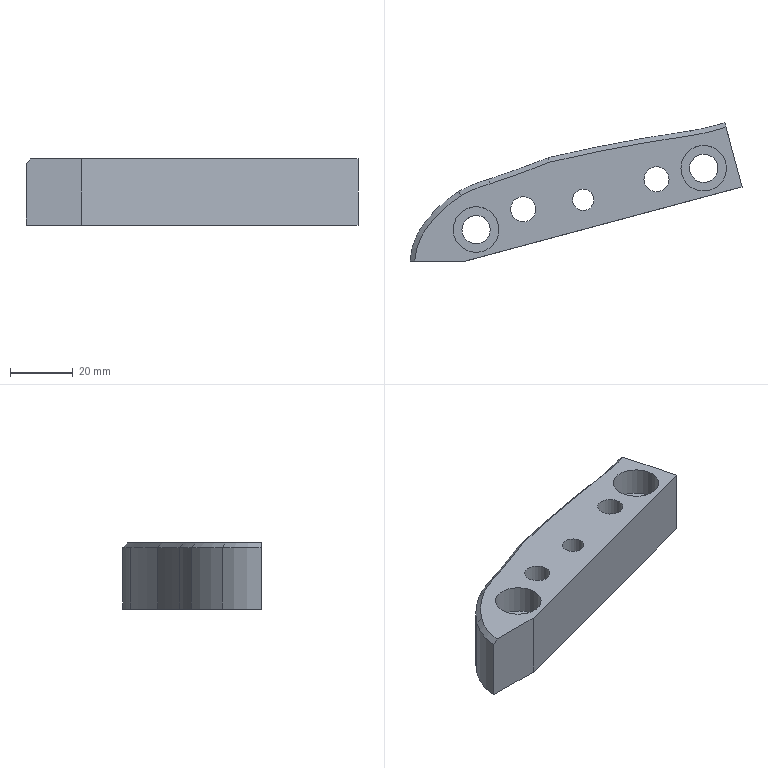Part | NX | features 23 2 | 1 solid | 26 faces | box 105.513 x 43.92 x 21 mm | volume 41296 mm3 | cylinder 13 | plane 7 | cone 6 | commonest cylinder face diameters 8.001 x2 9 x2 14.5 x2 6.8 x1 42.851 x1 79.35 x1
STEP:
#1=CARTESIAN_POINT('',(1132.197,150.506,-2.5));
#2=VERTEX_POINT('',#1);
#3=CARTESIAN_POINT('',(1124.947,150.506,-2.5));
#4=DIRECTION('',(0.,0.,1.));
#5=DIRECTION('',(1.,0.,0.));
#6=AXIS2_PLACEMENT_3D('',#3,#4,#5);
#7=CIRCLE('',#6,7.25);
#8=EDGE_CURVE('',#2,#2,#7,.T.);
#9=ORIENTED_EDGE('',*,*,#8,.F.);
#10=EDGE_LOOP('',(#9));
#11=FACE_BOUND('',#10,.T.);
#12=CARTESIAN_POINT('',(1113.947,147.035,-2.5));
#13=VERTEX_POINT('',#12);
#14=CARTESIAN_POINT('',(1109.947,147.035,-2.5));
#15=DIRECTION('',(0.,0.,-1.));
#16=DIRECTION('',(1.,0.,0.));
#17=AXIS2_PLACEMENT_3D('',#14,#15,#16);
#18=CIRCLE('',#17,4.);
#19=EDGE_CURVE('',#13,#13,#18,.T.);
#20=ORIENTED_EDGE('',*,*,#19,.T.);
#21=EDGE_LOOP('',(#20));
#22=FACE_BOUND('',#21,.T.);
#23=CARTESIAN_POINT('',(1071.605,137.506,-2.5));
#24=VERTEX_POINT('',#23);
#25=CARTESIAN_POINT('',(1067.604,137.506,-2.5));
#26=DIRECTION('',(0.,0.,-1.));
#27=DIRECTION('',(1.,0.,0.));
#28=AXIS2_PLACEMENT_3D('',#25,#26,#27);
#29=CIRCLE('',#28,4.);
#30=EDGE_CURVE('',#24,#24,#29,.T.);
#31=ORIENTED_EDGE('',*,*,#30,.T.);
#32=EDGE_LOOP('',(#31));
#33=FACE_BOUND('',#32,.T.);
#34=CARTESIAN_POINT('',(1059.854,131.035,-2.5));
#35=VERTEX_POINT('',#34);
#36=CARTESIAN_POINT('',(1052.604,131.035,-2.5));
#37=DIRECTION('',(0.,0.,1.));
#38=DIRECTION('',(1.,0.,0.));
#39=AXIS2_PLACEMENT_3D('',#36,#37,#38);
#40=CIRCLE('',#39,7.25);
#41=EDGE_CURVE('',#35,#35,#40,.T.);
#42=ORIENTED_EDGE('',*,*,#41,.F.);
#43=EDGE_LOOP('',(#42));
#44=FACE_BOUND('',#43,.T.);
#45=CARTESIAN_POINT('',(1132.046,163.506,-2.5));
#46=VERTEX_POINT('',#45);
#47=CARTESIAN_POINT('',(1137.117,144.58,-2.5));
#48=VERTEX_POINT('',#47);
#49=CARTESIAN_POINT('',(1105.356,263.116,-2.5));
#50=DIRECTION('',(0.2588,-0.9659,0.));
#51=VECTOR('',#50,1000.);
#52=LINE('',#49,#51);
#53=EDGE_CURVE('',#46,#48,#52,.T.);
#54=ORIENTED_EDGE('',*,*,#53,.F.);
#55=CARTESIAN_POINT('',(1120.988,160.941,-2.5));
#56=VERTEX_POINT('',#55);
#57=CARTESIAN_POINT('',(1105.089,254.594,-2.5));
#58=DIRECTION('',(0.,0.,1.));
#59=DIRECTION('',(1.,0.,0.));
#60=AXIS2_PLACEMENT_3D('',#57,#58,#59);
#61=CIRCLE('',#60,94.993);
#62=EDGE_CURVE('',#56,#46,#61,.T.);
#63=ORIENTED_EDGE('',*,*,#62,.F.);
#64=CARTESIAN_POINT('',(1075.995,152.47,-2.5));
#65=VERTEX_POINT('',#64);
#66=CARTESIAN_POINT('',(1196.799,-365.438,-2.5));
#67=DIRECTION('',(0.,0.,1.));
#68=DIRECTION('',(1.,0.,0.));
#69=AXIS2_PLACEMENT_3D('',#66,#67,#68);
#70=CIRCLE('',#69,531.81);
#71=EDGE_CURVE('',#56,#65,#70,.T.);
#72=ORIENTED_EDGE('',*,*,#71,.T.);
#73=CARTESIAN_POINT('',(1057.073,145.621,-2.5));
#74=VERTEX_POINT('',#73);
#75=CARTESIAN_POINT('',(961.955,437.965,-2.5));
#76=DIRECTION('',(0.,0.,1.));
#77=DIRECTION('',(1.,0.,0.));
#78=AXIS2_PLACEMENT_3D('',#75,#76,#77);
#79=CIRCLE('',#78,307.429);
#80=EDGE_CURVE('',#74,#65,#79,.T.);
#81=ORIENTED_EDGE('',*,*,#80,.F.);
#82=CARTESIAN_POINT('',(1047.857,141.866,-2.5));
#83=VERTEX_POINT('',#82);
#84=CARTESIAN_POINT('',(1069.196,102.677,-2.5));
#85=DIRECTION('',(0.,0.,1.));
#86=DIRECTION('',(1.,0.,0.));
#87=AXIS2_PLACEMENT_3D('',#84,#85,#86);
#88=CIRCLE('',#87,44.622);
#89=EDGE_CURVE('',#74,#83,#88,.T.);
#90=ORIENTED_EDGE('',*,*,#89,.T.);
#91=CARTESIAN_POINT('',(1037.481,132.386,-2.5));
#92=VERTEX_POINT('',#91);
#93=CARTESIAN_POINT('',(1067.977,109.423,-2.5));
#94=DIRECTION('',(0.,0.,1.));
#95=DIRECTION('',(1.,0.,0.));
#96=AXIS2_PLACEMENT_3D('',#93,#94,#95);
#97=CIRCLE('',#96,38.175);
#98=EDGE_CURVE('',#83,#92,#97,.T.);
#99=ORIENTED_EDGE('',*,*,#98,.T.);
#100=CARTESIAN_POINT('',(1033.106,121.035,-2.5));
#101=VERTEX_POINT('',#100);
#102=CARTESIAN_POINT('',(1052.999,119.888,-2.5));
#103=DIRECTION('',(0.,0.,1.));
#104=DIRECTION('',(1.,0.,0.));
#105=AXIS2_PLACEMENT_3D('',#102,#103,#104);
#106=CIRCLE('',#105,19.925);
#107=EDGE_CURVE('',#92,#101,#106,.T.);
#108=ORIENTED_EDGE('',*,*,#107,.T.);
#109=CARTESIAN_POINT('',(1049.246,121.035,-2.5));
#110=VERTEX_POINT('',#109);
#111=CARTESIAN_POINT('',(1049.246,121.035,-2.5));
#112=DIRECTION('',(1.,0.,0.));
#113=VECTOR('',#112,1000.);
#114=LINE('',#111,#113);
#115=EDGE_CURVE('',#101,#110,#114,.T.);
#116=ORIENTED_EDGE('',*,*,#115,.T.);
#117=CARTESIAN_POINT('',(1110.705,137.503,-2.5));
#118=DIRECTION('',(0.9659,0.2588,0.));
#119=VECTOR('',#118,1000.);
#120=LINE('',#117,#119);
#121=EDGE_CURVE('',#110,#48,#120,.T.);
#122=ORIENTED_EDGE('',*,*,#121,.T.);
#123=EDGE_LOOP('',(#54,#63,#72,#81,#90,#99,#108,#116,#122));
#124=FACE_BOUND('',#123,.T.);
#125=CARTESIAN_POINT('',(1090.03,140.472,-2.5));
#126=VERTEX_POINT('',#125);
#127=CARTESIAN_POINT('',(1086.63,140.472,-2.5));
#128=DIRECTION('',(0.,0.,1.));
#129=DIRECTION('',(1.,0.,0.));
#130=AXIS2_PLACEMENT_3D('',#127,#128,#129);
#131=CIRCLE('',#130,3.4);
#132=EDGE_CURVE('',#126,#126,#131,.T.);
#133=ORIENTED_EDGE('',*,*,#132,.F.);
#134=EDGE_LOOP('',(#133));
#135=FACE_BOUND('',#134,.T.);
#136=CARTESIAN_POINT('',(1166.5,279.5,-2.5));
#137=DIRECTION('',(0.,0.,1.));
#138=DIRECTION('',(-1.,0.,0.));
#139=AXIS2_PLACEMENT_3D('',#136,#137,#138);
#140=PLANE('',#139);
#141=ADVANCED_FACE('',(#11,#22,#33,#44,#124,#135),#140,.T.);
#142=CARTESIAN_POINT('',(1137.117,144.58,-23.5));
#143=VERTEX_POINT('',#142);
#144=CARTESIAN_POINT('',(1137.117,144.58,-33.5));
#145=DIRECTION('',(0.,0.,-1.));
#146=VECTOR('',#145,1000.);
#147=LINE('',#144,#146);
#148=EDGE_CURVE('',#48,#143,#147,.T.);
#149=ORIENTED_EDGE('',*,*,#148,.F.);
#150=ORIENTED_EDGE('',*,*,#121,.F.);
#151=CARTESIAN_POINT('',(1049.246,121.035,-23.5));
#152=VERTEX_POINT('',#151);
#153=CARTESIAN_POINT('',(1049.246,121.035,-33.5));
#154=DIRECTION('',(0.,0.,1.));
#155=VECTOR('',#154,1000.);
#156=LINE('',#153,#155);
#157=EDGE_CURVE('',#152,#110,#156,.T.);
#158=ORIENTED_EDGE('',*,*,#157,.F.);
#159=CARTESIAN_POINT('',(1110.705,137.503,-23.5));
#160=DIRECTION('',(-0.9659,-0.2588,0.));
#161=VECTOR('',#160,1000.);
#162=LINE('',#159,#161);
#163=EDGE_CURVE('',#143,#152,#162,.T.);
#164=ORIENTED_EDGE('',*,*,#163,.F.);
#165=EDGE_LOOP('',(#149,#150,#158,#164));
#166=FACE_BOUND('',#165,.T.);
#167=CARTESIAN_POINT('',(1110.705,137.503,-33.5));
#168=DIRECTION('',(0.2588,-0.9659,0.));
#169=DIRECTION('',(0.,0.,-1.));
#170=AXIS2_PLACEMENT_3D('',#167,#168,#169);
#171=PLANE('',#170);
#172=ADVANCED_FACE('',(#166),#171,.T.);
#173=CARTESIAN_POINT('',(1075.544,153.905,-4.));
#174=VERTEX_POINT('',#173);
#175=CARTESIAN_POINT('',(1076.1,152.135,-2.15));
#176=CARTESIAN_POINT('',(1076.077,152.209,-2.227));
#177=CARTESIAN_POINT('',(1076.054,152.282,-2.304));
#178=CARTESIAN_POINT('',(1076.013,152.413,-2.44));
#179=CARTESIAN_POINT('',(1075.995,152.469,-2.499));
#180=CARTESIAN_POINT('',(1075.964,152.569,-2.604));
#181=CARTESIAN_POINT('',(1075.95,152.613,-2.649));
#182=CARTESIAN_POINT('',(1075.926,152.69,-2.73));
#183=CARTESIAN_POINT('',(1075.915,152.723,-2.765));
#184=CARTESIAN_POINT('',(1075.835,152.98,-3.033));
#185=CARTESIAN_POINT('',(1075.764,153.203,-3.267));
#186=CARTESIAN_POINT('',(1075.684,153.46,-3.535));
#187=CARTESIAN_POINT('',(1075.673,153.493,-3.57));
#188=CARTESIAN_POINT('',(1075.649,153.57,-3.65));
#189=CARTESIAN_POINT('',(1075.635,153.614,-3.696));
#190=CARTESIAN_POINT('',(1075.604,153.714,-3.801));
#191=CARTESIAN_POINT('',(1075.586,153.771,-3.86));
#192=CARTESIAN_POINT('',(1075.545,153.901,-3.996));
#193=CARTESIAN_POINT('',(1075.522,153.974,-4.073));
#194=CARTESIAN_POINT('',(1075.499,154.048,-4.15));
#195=B_SPLINE_CURVE_WITH_KNOTS('',3,(#175,#176,#177,#178,#179,#180,#181,#182,#183,#184,#185,#186,#187,#188,#189,#190,#191,#192,#193,#194),.UNSPECIFIED.,.F.,.F.,(4,2,2,2,2,2,2,2,2,4),(0.,0.1154,0.2041,0.2724,0.3249,0.6751,0.7276,0.7959,0.8846,1.),.UNSPECIFIED.);
#196=EDGE_CURVE('',#65,#174,#195,.T.);
#197=ORIENTED_EDGE('',*,*,#196,.F.);
#198=ORIENTED_EDGE('',*,*,#71,.F.);
#199=CARTESIAN_POINT('',(1120.756,162.423,-4.));
#200=VERTEX_POINT('',#199);
#201=CARTESIAN_POINT('',(1121.042,160.595,-2.15));
#202=CARTESIAN_POINT('',(1121.03,160.671,-2.227));
#203=CARTESIAN_POINT('',(1121.018,160.747,-2.304));
#204=CARTESIAN_POINT('',(1120.997,160.882,-2.44));
#205=CARTESIAN_POINT('',(1120.988,160.94,-2.499));
#206=CARTESIAN_POINT('',(1120.972,161.044,-2.604));
#207=CARTESIAN_POINT('',(1120.965,161.089,-2.649));
#208=CARTESIAN_POINT('',(1120.952,161.168,-2.73));
#209=CARTESIAN_POINT('',(1120.947,161.203,-2.765));
#210=CARTESIAN_POINT('',(1120.905,161.468,-3.033));
#211=CARTESIAN_POINT('',(1120.869,161.698,-3.267));
#212=CARTESIAN_POINT('',(1120.828,161.963,-3.535));
#213=CARTESIAN_POINT('',(1120.822,161.998,-3.57));
#214=CARTESIAN_POINT('',(1120.81,162.078,-3.65));
#215=CARTESIAN_POINT('',(1120.803,162.123,-3.696));
#216=CARTESIAN_POINT('',(1120.786,162.226,-3.801));
#217=CARTESIAN_POINT('',(1120.777,162.284,-3.86));
#218=CARTESIAN_POINT('',(1120.756,162.419,-3.996));
#219=CARTESIAN_POINT('',(1120.744,162.495,-4.073));
#220=CARTESIAN_POINT('',(1120.732,162.571,-4.15));
#221=B_SPLINE_CURVE_WITH_KNOTS('',3,(#201,#202,#203,#204,#205,#206,#207,#208,#209,#210,#211,#212,#213,#214,#215,#216,#217,#218,#219,#220),.UNSPECIFIED.,.F.,.F.,(4,2,2,2,2,2,2,2,2,4),(0.,0.1154,0.2041,0.2724,0.3249,0.6751,0.7276,0.7959,0.8846,1.),.UNSPECIFIED.);
#222=EDGE_CURVE('',#56,#200,#221,.T.);
#223=ORIENTED_EDGE('',*,*,#222,.T.);
#224=CARTESIAN_POINT('',(1196.799,-365.438,-4.));
#225=DIRECTION('',(0.,0.,-1.));
#226=DIRECTION('',(-1.,0.,0.));
#227=AXIS2_PLACEMENT_3D('',#224,#225,#226);
#228=CIRCLE('',#227,533.31);
#229=EDGE_CURVE('',#174,#200,#228,.T.);
#230=ORIENTED_EDGE('',*,*,#229,.F.);
#231=EDGE_LOOP('',(#197,#198,#223,#230));
#232=FACE_BOUND('',#231,.T.);
#233=CARTESIAN_POINT('',(1196.799,-365.438,-3.5));
#234=DIRECTION('',(0.,0.,-1.));
#235=DIRECTION('',(-1.,0.,0.));
#236=AXIS2_PLACEMENT_3D('',#233,#234,#235);
#237=CONICAL_SURFACE('',#236,532.81,0.7854);
#238=ADVANCED_FACE('',(#232),#237,.T.);
#239=ORIENTED_EDGE('',*,*,#80,.T.);
#240=ORIENTED_EDGE('',*,*,#196,.T.);
#241=CARTESIAN_POINT('',(1056.637,147.056,-4.));
#242=VERTEX_POINT('',#241);
#243=CARTESIAN_POINT('',(961.955,437.965,-4.));
#244=DIRECTION('',(0.,0.,-1.));
#245=DIRECTION('',(1.,0.,0.));
#246=AXIS2_PLACEMENT_3D('',#243,#244,#245);
#247=CIRCLE('',#246,305.929);
#248=EDGE_CURVE('',#174,#242,#247,.T.);
#249=ORIENTED_EDGE('',*,*,#248,.T.);
#250=CARTESIAN_POINT('',(1057.175,145.286,-2.15));
#251=CARTESIAN_POINT('',(1057.152,145.36,-2.227));
#252=CARTESIAN_POINT('',(1057.13,145.433,-2.304));
#253=CARTESIAN_POINT('',(1057.09,145.563,-2.44));
#254=CARTESIAN_POINT('',(1057.073,145.62,-2.499));
#255=CARTESIAN_POINT('',(1057.043,145.72,-2.604));
#256=CARTESIAN_POINT('',(1057.03,145.764,-2.65));
#257=CARTESIAN_POINT('',(1057.006,145.841,-2.73));
#258=CARTESIAN_POINT('',(1056.996,145.874,-2.765));
#259=CARTESIAN_POINT('',(1056.918,146.131,-3.033));
#260=CARTESIAN_POINT('',(1056.85,146.354,-3.267));
#261=CARTESIAN_POINT('',(1056.772,146.611,-3.535));
#262=CARTESIAN_POINT('',(1056.762,146.645,-3.57));
#263=CARTESIAN_POINT('',(1056.738,146.722,-3.651));
#264=CARTESIAN_POINT('',(1056.725,146.765,-3.696));
#265=CARTESIAN_POINT('',(1056.695,146.865,-3.801));
#266=CARTESIAN_POINT('',(1056.678,146.922,-3.86));
#267=CARTESIAN_POINT('',(1056.638,147.052,-3.996));
#268=CARTESIAN_POINT('',(1056.616,147.126,-4.073));
#269=CARTESIAN_POINT('',(1056.593,147.199,-4.15));
#270=B_SPLINE_CURVE_WITH_KNOTS('',3,(#250,#251,#252,#253,#254,#255,#256,#257,#258,#259,#260,#261,#262,#263,#264,#265,#266,#267,#268,#269),.UNSPECIFIED.,.F.,.F.,(4,2,2,2,2,2,2,2,2,4),(0.,0.1154,0.2041,0.2724,0.3249,0.6751,0.7276,0.7959,0.8846,1.),.UNSPECIFIED.);
#271=EDGE_CURVE('',#74,#242,#270,.T.);
#272=ORIENTED_EDGE('',*,*,#271,.F.);
#273=EDGE_LOOP('',(#239,#240,#249,#272));
#274=FACE_BOUND('',#273,.T.);
#275=CARTESIAN_POINT('',(961.955,437.965,-3.5));
#276=DIRECTION('',(0.,0.,1.));
#277=DIRECTION('',(1.,0.,0.));
#278=AXIS2_PLACEMENT_3D('',#275,#276,#277);
#279=CONICAL_SURFACE('',#278,306.429,0.7854);
#280=ADVANCED_FACE('',(#274),#279,.F.);
#281=CARTESIAN_POINT('',(1047.102,143.163,-4.));
#282=VERTEX_POINT('',#281);
#283=CARTESIAN_POINT('',(1047.027,143.292,-4.15));
#284=CARTESIAN_POINT('',(1047.065,143.226,-4.073));
#285=CARTESIAN_POINT('',(1047.104,143.159,-3.996));
#286=CARTESIAN_POINT('',(1047.173,143.041,-3.86));
#287=CARTESIAN_POINT('',(1047.202,142.99,-3.801));
#288=CARTESIAN_POINT('',(1047.255,142.9,-3.696));
#289=CARTESIAN_POINT('',(1047.278,142.86,-3.651));
#290=CARTESIAN_POINT('',(1047.318,142.791,-3.57));
#291=CARTESIAN_POINT('',(1047.336,142.761,-3.535));
#292=CARTESIAN_POINT('',(1047.471,142.529,-3.267));
#293=CARTESIAN_POINT('',(1047.588,142.327,-3.033));
#294=CARTESIAN_POINT('',(1047.723,142.095,-2.765));
#295=CARTESIAN_POINT('',(1047.741,142.064,-2.73));
#296=CARTESIAN_POINT('',(1047.781,141.995,-2.65));
#297=CARTESIAN_POINT('',(1047.804,141.955,-2.604));
#298=CARTESIAN_POINT('',(1047.857,141.865,-2.499));
#299=CARTESIAN_POINT('',(1047.887,141.814,-2.44));
#300=CARTESIAN_POINT('',(1047.955,141.696,-2.304));
#301=CARTESIAN_POINT('',(1047.994,141.63,-2.227));
#302=CARTESIAN_POINT('',(1048.032,141.563,-2.15));
#303=B_SPLINE_CURVE_WITH_KNOTS('',3,(#283,#284,#285,#286,#287,#288,#289,#290,#291,#292,#293,#294,#295,#296,#297,#298,#299,#300,#301,#302),.UNSPECIFIED.,.F.,.F.,(4,2,2,2,2,2,2,2,2,4),(0.,0.1154,0.2041,0.2724,0.3249,0.6751,0.7276,0.7959,0.8846,1.),.UNSPECIFIED.);
#304=EDGE_CURVE('',#282,#83,#303,.T.);
#305=ORIENTED_EDGE('',*,*,#304,.T.);
#306=ORIENTED_EDGE('',*,*,#89,.F.);
#307=ORIENTED_EDGE('',*,*,#271,.T.);
#308=CARTESIAN_POINT('',(1069.196,102.677,-4.));
#309=DIRECTION('',(0.,0.,-1.));
#310=DIRECTION('',(-1.,0.,0.));
#311=AXIS2_PLACEMENT_3D('',#308,#309,#310);
#312=CIRCLE('',#311,46.122);
#313=EDGE_CURVE('',#282,#242,#312,.T.);
#314=ORIENTED_EDGE('',*,*,#313,.F.);
#315=EDGE_LOOP('',(#305,#306,#307,#314));
#316=FACE_BOUND('',#315,.T.);
#317=CARTESIAN_POINT('',(1069.196,102.677,-3.5));
#318=DIRECTION('',(0.,0.,-1.));
#319=DIRECTION('',(-1.,0.,0.));
#320=AXIS2_PLACEMENT_3D('',#317,#318,#319);
#321=CONICAL_SURFACE('',#320,45.622,0.7854);
#322=ADVANCED_FACE('',(#316),#321,.T.);
#323=CARTESIAN_POINT('',(1031.604,121.035,-4.));
#324=VERTEX_POINT('',#323);
#325=CARTESIAN_POINT('',(1031.604,121.035,-4.));
#326=CARTESIAN_POINT('',(1031.932,121.035,-3.673));
#327=CARTESIAN_POINT('',(1032.26,121.035,-3.345));
#328=CARTESIAN_POINT('',(1032.761,121.035,-2.845));
#329=CARTESIAN_POINT('',(1032.933,121.035,-2.673));
#330=CARTESIAN_POINT('',(1033.106,121.035,-2.5));
#331=B_SPLINE_CURVE_WITH_KNOTS('',3,(#325,#326,#327,#328,#329,#330),.UNSPECIFIED.,.F.,.F.,(4,2,4),(0.,0.6548,1.),.UNSPECIFIED.);
#332=EDGE_CURVE('',#324,#101,#331,.T.);
#333=ORIENTED_EDGE('',*,*,#332,.T.);
#334=ORIENTED_EDGE('',*,*,#107,.F.);
#335=CARTESIAN_POINT('',(1036.297,133.308,-4.));
#336=VERTEX_POINT('',#335);
#337=CARTESIAN_POINT('',(1036.179,133.4,-4.15));
#338=CARTESIAN_POINT('',(1036.24,133.353,-4.073));
#339=CARTESIAN_POINT('',(1036.3,133.306,-3.996));
#340=CARTESIAN_POINT('',(1036.408,133.222,-3.86));
#341=CARTESIAN_POINT('',(1036.454,133.186,-3.801));
#342=CARTESIAN_POINT('',(1036.537,133.121,-3.696));
#343=CARTESIAN_POINT('',(1036.573,133.093,-3.651));
#344=CARTESIAN_POINT('',(1036.636,133.044,-3.57));
#345=CARTESIAN_POINT('',(1036.664,133.022,-3.535));
#346=CARTESIAN_POINT('',(1036.876,132.858,-3.267));
#347=CARTESIAN_POINT('',(1037.06,132.714,-3.033));
#348=CARTESIAN_POINT('',(1037.272,132.549,-2.765));
#349=CARTESIAN_POINT('',(1037.299,132.528,-2.73));
#350=CARTESIAN_POINT('',(1037.363,132.478,-2.65));
#351=CARTESIAN_POINT('',(1037.399,132.45,-2.604));
#352=CARTESIAN_POINT('',(1037.481,132.386,-2.499));
#353=CARTESIAN_POINT('',(1037.528,132.35,-2.44));
#354=CARTESIAN_POINT('',(1037.635,132.266,-2.304));
#355=CARTESIAN_POINT('',(1037.696,132.219,-2.227));
#356=CARTESIAN_POINT('',(1037.757,132.172,-2.15));
#357=B_SPLINE_CURVE_WITH_KNOTS('',3,(#337,#338,#339,#340,#341,#342,#343,#344,#345,#346,#347,#348,#349,#350,#351,#352,#353,#354,#355,#356),.UNSPECIFIED.,.F.,.F.,(4,2,2,2,2,2,2,2,2,4),(0.,0.1154,0.2041,0.2724,0.3249,0.6751,0.7276,0.7959,0.8846,1.),.UNSPECIFIED.);
#358=EDGE_CURVE('',#336,#92,#357,.T.);
#359=ORIENTED_EDGE('',*,*,#358,.F.);
#360=CARTESIAN_POINT('',(1052.999,119.888,-4.));
#361=DIRECTION('',(0.,0.,-1.));
#362=DIRECTION('',(-1.,0.,0.));
#363=AXIS2_PLACEMENT_3D('',#360,#361,#362);
#364=CIRCLE('',#363,21.425);
#365=EDGE_CURVE('',#324,#336,#364,.T.);
#366=ORIENTED_EDGE('',*,*,#365,.F.);
#367=EDGE_LOOP('',(#333,#334,#359,#366));
#368=FACE_BOUND('',#367,.T.);
#369=CARTESIAN_POINT('',(1052.999,119.888,-3.5));
#370=DIRECTION('',(0.,0.,-1.));
#371=DIRECTION('',(-1.,0.,0.));
#372=AXIS2_PLACEMENT_3D('',#369,#370,#371);
#373=CONICAL_SURFACE('',#372,20.925,0.7854);
#374=ADVANCED_FACE('',(#368),#373,.T.);
#375=ORIENTED_EDGE('',*,*,#358,.T.);
#376=ORIENTED_EDGE('',*,*,#98,.F.);
#377=ORIENTED_EDGE('',*,*,#304,.F.);
#378=CARTESIAN_POINT('',(1067.977,109.423,-4.));
#379=DIRECTION('',(0.,0.,-1.));
#380=DIRECTION('',(-1.,0.,0.));
#381=AXIS2_PLACEMENT_3D('',#378,#379,#380);
#382=CIRCLE('',#381,39.675);
#383=EDGE_CURVE('',#336,#282,#382,.T.);
#384=ORIENTED_EDGE('',*,*,#383,.F.);
#385=EDGE_LOOP('',(#375,#376,#377,#384));
#386=FACE_BOUND('',#385,.T.);
#387=CARTESIAN_POINT('',(1067.977,109.423,-3.5));
#388=DIRECTION('',(0.,0.,-1.));
#389=DIRECTION('',(-1.,0.,0.));
#390=AXIS2_PLACEMENT_3D('',#387,#388,#389);
#391=CONICAL_SURFACE('',#390,39.175,0.7854);
#392=ADVANCED_FACE('',(#386),#391,.T.);
#393=ORIENTED_EDGE('',*,*,#332,.F.);
#394=CARTESIAN_POINT('',(1031.604,121.035,-23.5));
#395=VERTEX_POINT('',#394);
#396=CARTESIAN_POINT('',(1031.604,121.035,-43.));
#397=DIRECTION('',(0.,0.,-1.));
#398=VECTOR('',#397,1000.);
#399=LINE('',#396,#398);
#400=EDGE_CURVE('',#324,#395,#399,.T.);
#401=ORIENTED_EDGE('',*,*,#400,.T.);
#402=CARTESIAN_POINT('',(1084.824,121.035,-23.5));
#403=DIRECTION('',(1.,0.,0.));
#404=VECTOR('',#403,1000.);
#405=LINE('',#402,#404);
#406=EDGE_CURVE('',#395,#152,#405,.T.);
#407=ORIENTED_EDGE('',*,*,#406,.T.);
#408=ORIENTED_EDGE('',*,*,#157,.T.);
#409=ORIENTED_EDGE('',*,*,#115,.F.);
#410=EDGE_LOOP('',(#393,#401,#407,#408,#409));
#411=FACE_BOUND('',#410,.T.);
#412=CARTESIAN_POINT('',(1049.246,121.035,-3.5));
#413=DIRECTION('',(0.,-1.,0.));
#414=DIRECTION('',(0.,0.,1.));
#415=AXIS2_PLACEMENT_3D('',#412,#413,#414);
#416=PLANE('',#415);
#417=ADVANCED_FACE('',(#411),#416,.T.);
#418=CARTESIAN_POINT('',(1083.23,140.472,-23.5));
#419=VERTEX_POINT('',#418);
#420=CARTESIAN_POINT('',(1086.63,140.472,-23.5));
#421=DIRECTION('',(0.,0.,1.));
#422=DIRECTION('',(-1.,0.,0.));
#423=AXIS2_PLACEMENT_3D('',#420,#421,#422);
#424=CIRCLE('',#423,3.4);
#425=EDGE_CURVE('',#419,#419,#424,.T.);
#426=ORIENTED_EDGE('',*,*,#425,.T.);
#427=EDGE_LOOP('',(#426));
#428=FACE_BOUND('',#427,.T.);
#429=CARTESIAN_POINT('',(1131.658,164.955,-23.5));
#430=VERTEX_POINT('',#429);
#431=CARTESIAN_POINT('',(1111.235,241.173,-23.5));
#432=DIRECTION('',(-0.2588,0.9659,0.));
#433=VECTOR('',#432,1000.);
#434=LINE('',#431,#433);
#435=EDGE_CURVE('',#143,#430,#434,.T.);
#436=ORIENTED_EDGE('',*,*,#435,.F.);
#437=ORIENTED_EDGE('',*,*,#163,.T.);
#438=ORIENTED_EDGE('',*,*,#406,.F.);
#439=CARTESIAN_POINT('',(1036.297,133.308,-23.5));
#440=VERTEX_POINT('',#439);
#441=CARTESIAN_POINT('',(1052.999,119.888,-23.5));
#442=DIRECTION('',(0.,0.,1.));
#443=DIRECTION('',(-1.,0.,0.));
#444=AXIS2_PLACEMENT_3D('',#441,#442,#443);
#445=CIRCLE('',#444,21.425);
#446=EDGE_CURVE('',#440,#395,#445,.T.);
#447=ORIENTED_EDGE('',*,*,#446,.F.);
#448=CARTESIAN_POINT('',(1047.102,143.163,-23.5));
#449=VERTEX_POINT('',#448);
#450=CARTESIAN_POINT('',(1067.977,109.423,-23.5));
#451=DIRECTION('',(0.,0.,1.));
#452=DIRECTION('',(-1.,0.,0.));
#453=AXIS2_PLACEMENT_3D('',#450,#451,#452);
#454=CIRCLE('',#453,39.675);
#455=EDGE_CURVE('',#449,#440,#454,.T.);
#456=ORIENTED_EDGE('',*,*,#455,.F.);
#457=CARTESIAN_POINT('',(1056.637,147.056,-23.5));
#458=VERTEX_POINT('',#457);
#459=CARTESIAN_POINT('',(1069.196,102.677,-23.5));
#460=DIRECTION('',(0.,0.,-1.));
#461=DIRECTION('',(-1.,0.,0.));
#462=AXIS2_PLACEMENT_3D('',#459,#460,#461);
#463=CIRCLE('',#462,46.122);
#464=EDGE_CURVE('',#449,#458,#463,.T.);
#465=ORIENTED_EDGE('',*,*,#464,.T.);
#466=CARTESIAN_POINT('',(1075.544,153.905,-23.5));
#467=VERTEX_POINT('',#466);
#468=CARTESIAN_POINT('',(961.955,437.965,-23.5));
#469=DIRECTION('',(0.,0.,1.));
#470=DIRECTION('',(-1.,0.,0.));
#471=AXIS2_PLACEMENT_3D('',#468,#469,#470);
#472=CIRCLE('',#471,305.929);
#473=EDGE_CURVE('',#458,#467,#472,.T.);
#474=ORIENTED_EDGE('',*,*,#473,.T.);
#475=CARTESIAN_POINT('',(1120.756,162.423,-23.5));
#476=VERTEX_POINT('',#475);
#477=CARTESIAN_POINT('',(1196.799,-365.438,-23.5));
#478=DIRECTION('',(0.,0.,1.));
#479=DIRECTION('',(-1.,0.,0.));
#480=AXIS2_PLACEMENT_3D('',#477,#478,#479);
#481=CIRCLE('',#480,533.31);
#482=EDGE_CURVE('',#476,#467,#481,.T.);
#483=ORIENTED_EDGE('',*,*,#482,.F.);
#484=CARTESIAN_POINT('',(1105.089,254.594,-23.5));
#485=DIRECTION('',(0.,0.,1.));
#486=DIRECTION('',(-1.,0.,0.));
#487=AXIS2_PLACEMENT_3D('',#484,#485,#486);
#488=CIRCLE('',#487,93.493);
#489=EDGE_CURVE('',#476,#430,#488,.T.);
#490=ORIENTED_EDGE('',*,*,#489,.T.);
#491=EDGE_LOOP('',(#436,#437,#438,#447,#456,#465,#474,#483,#490));
#492=FACE_BOUND('',#491,.T.);
#493=CARTESIAN_POINT('',(1120.447,150.506,-23.5));
#494=VERTEX_POINT('',#493);
#495=CARTESIAN_POINT('',(1124.947,150.506,-23.5));
#496=DIRECTION('',(0.,0.,1.));
#497=DIRECTION('',(-1.,0.,0.));
#498=AXIS2_PLACEMENT_3D('',#495,#496,#497);
#499=CIRCLE('',#498,4.5);
#500=EDGE_CURVE('',#494,#494,#499,.T.);
#501=ORIENTED_EDGE('',*,*,#500,.T.);
#502=EDGE_LOOP('',(#501));
#503=FACE_BOUND('',#502,.T.);
#504=CARTESIAN_POINT('',(1048.104,131.035,-23.5));
#505=VERTEX_POINT('',#504);
#506=CARTESIAN_POINT('',(1052.604,131.035,-23.5));
#507=DIRECTION('',(0.,0.,1.));
#508=DIRECTION('',(-1.,0.,0.));
#509=AXIS2_PLACEMENT_3D('',#506,#507,#508);
#510=CIRCLE('',#509,4.5);
#511=EDGE_CURVE('',#505,#505,#510,.T.);
#512=ORIENTED_EDGE('',*,*,#511,.T.);
#513=EDGE_LOOP('',(#512));
#514=FACE_BOUND('',#513,.T.);
#515=CARTESIAN_POINT('',(1063.604,137.506,-23.5));
#516=VERTEX_POINT('',#515);
#517=CARTESIAN_POINT('',(1067.604,137.506,-23.5));
#518=DIRECTION('',(0.,0.,1.));
#519=DIRECTION('',(-1.,0.,0.));
#520=AXIS2_PLACEMENT_3D('',#517,#518,#519);
#521=CIRCLE('',#520,4.);
#522=EDGE_CURVE('',#516,#516,#521,.T.);
#523=ORIENTED_EDGE('',*,*,#522,.T.);
#524=EDGE_LOOP('',(#523));
#525=FACE_BOUND('',#524,.T.);
#526=CARTESIAN_POINT('',(1105.946,147.035,-23.5));
#527=VERTEX_POINT('',#526);
#528=CARTESIAN_POINT('',(1109.947,147.035,-23.5));
#529=DIRECTION('',(0.,0.,1.));
#530=DIRECTION('',(-1.,0.,0.));
#531=AXIS2_PLACEMENT_3D('',#528,#529,#530);
#532=CIRCLE('',#531,4.);
#533=EDGE_CURVE('',#527,#527,#532,.T.);
#534=ORIENTED_EDGE('',*,*,#533,.T.);
#535=EDGE_LOOP('',(#534));
#536=FACE_BOUND('',#535,.T.);
#537=CARTESIAN_POINT('',(1084.824,234.096,-23.5));
#538=DIRECTION('',(0.,0.,-1.));
#539=DIRECTION('',(-0.2588,0.9659,0.));
#540=AXIS2_PLACEMENT_3D('',#537,#538,#539);
#541=PLANE('',#540);
#542=ADVANCED_FACE('',(#428,#492,#503,#514,#525,#536),#541,.T.);
#543=ORIENTED_EDGE('',*,*,#473,.F.);
#544=CARTESIAN_POINT('',(1056.637,147.056,-43.));
#545=DIRECTION('',(0.,0.,-1.));
#546=VECTOR('',#545,1000.);
#547=LINE('',#544,#546);
#548=EDGE_CURVE('',#242,#458,#547,.T.);
#549=ORIENTED_EDGE('',*,*,#548,.F.);
#550=ORIENTED_EDGE('',*,*,#248,.F.);
#551=CARTESIAN_POINT('',(1075.544,153.905,-43.));
#552=DIRECTION('',(0.,0.,-1.));
#553=VECTOR('',#552,1000.);
#554=LINE('',#551,#553);
#555=EDGE_CURVE('',#174,#467,#554,.T.);
#556=ORIENTED_EDGE('',*,*,#555,.T.);
#557=EDGE_LOOP('',(#543,#549,#550,#556));
#558=FACE_BOUND('',#557,.T.);
#559=CARTESIAN_POINT('',(961.955,437.965,-43.));
#560=DIRECTION('',(0.,0.,1.));
#561=DIRECTION('',(-1.,0.,0.));
#562=AXIS2_PLACEMENT_3D('',#559,#560,#561);
#563=CYLINDRICAL_SURFACE('',#562,305.929);
#564=ADVANCED_FACE('',(#558),#563,.F.);
#565=ORIENTED_EDGE('',*,*,#482,.T.);
#566=ORIENTED_EDGE('',*,*,#555,.F.);
#567=ORIENTED_EDGE('',*,*,#229,.T.);
#568=CARTESIAN_POINT('',(1120.756,162.423,-43.));
#569=DIRECTION('',(0.,0.,1.));
#570=VECTOR('',#569,1000.);
#571=LINE('',#568,#570);
#572=EDGE_CURVE('',#476,#200,#571,.T.);
#573=ORIENTED_EDGE('',*,*,#572,.F.);
#574=EDGE_LOOP('',(#565,#566,#567,#573));
#575=FACE_BOUND('',#574,.T.);
#576=CARTESIAN_POINT('',(1196.799,-365.438,-43.));
#577=DIRECTION('',(0.,0.,1.));
#578=DIRECTION('',(-1.,0.,0.));
#579=AXIS2_PLACEMENT_3D('',#576,#577,#578);
#580=CYLINDRICAL_SURFACE('',#579,533.31);
#581=ADVANCED_FACE('',(#575),#580,.T.);
#582=ORIENTED_EDGE('',*,*,#464,.F.);
#583=CARTESIAN_POINT('',(1047.102,143.163,-43.));
#584=DIRECTION('',(0.,0.,-1.));
#585=VECTOR('',#584,1000.);
#586=LINE('',#583,#585);
#587=EDGE_CURVE('',#282,#449,#586,.T.);
#588=ORIENTED_EDGE('',*,*,#587,.F.);
#589=ORIENTED_EDGE('',*,*,#313,.T.);
#590=ORIENTED_EDGE('',*,*,#548,.T.);
#591=EDGE_LOOP('',(#582,#588,#589,#590));
#592=FACE_BOUND('',#591,.T.);
#593=CARTESIAN_POINT('',(1069.196,102.677,-43.));
#594=DIRECTION('',(0.,0.,1.));
#595=DIRECTION('',(-1.,0.,0.));
#596=AXIS2_PLACEMENT_3D('',#593,#594,#595);
#597=CYLINDRICAL_SURFACE('',#596,46.122);
#598=ADVANCED_FACE('',(#592),#597,.T.);
#599=ORIENTED_EDGE('',*,*,#455,.T.);
#600=CARTESIAN_POINT('',(1036.297,133.308,-43.));
#601=DIRECTION('',(0.,0.,-1.));
#602=VECTOR('',#601,1000.);
#603=LINE('',#600,#602);
#604=EDGE_CURVE('',#336,#440,#603,.T.);
#605=ORIENTED_EDGE('',*,*,#604,.F.);
#606=ORIENTED_EDGE('',*,*,#383,.T.);
#607=ORIENTED_EDGE('',*,*,#587,.T.);
#608=EDGE_LOOP('',(#599,#605,#606,#607));
#609=FACE_BOUND('',#608,.T.);
#610=CARTESIAN_POINT('',(1067.977,109.423,-43.));
#611=DIRECTION('',(0.,0.,1.));
#612=DIRECTION('',(-1.,0.,0.));
#613=AXIS2_PLACEMENT_3D('',#610,#611,#612);
#614=CYLINDRICAL_SURFACE('',#613,39.675);
#615=ADVANCED_FACE('',(#609),#614,.T.);
#616=ORIENTED_EDGE('',*,*,#446,.T.);
#617=ORIENTED_EDGE('',*,*,#400,.F.);
#618=ORIENTED_EDGE('',*,*,#365,.T.);
#619=ORIENTED_EDGE('',*,*,#604,.T.);
#620=EDGE_LOOP('',(#616,#617,#618,#619));
#621=FACE_BOUND('',#620,.T.);
#622=CARTESIAN_POINT('',(1052.999,119.888,-43.));
#623=DIRECTION('',(0.,0.,1.));
#624=DIRECTION('',(-1.,0.,0.));
#625=AXIS2_PLACEMENT_3D('',#622,#623,#624);
#626=CYLINDRICAL_SURFACE('',#625,21.425);
#627=ADVANCED_FACE('',(#621),#626,.T.);
#628=CARTESIAN_POINT('',(1131.658,164.955,-4.));
#629=VERTEX_POINT('',#628);
#630=CARTESIAN_POINT('',(1105.089,254.594,-4.));
#631=DIRECTION('',(0.,0.,1.));
#632=DIRECTION('',(-1.,0.,0.));
#633=AXIS2_PLACEMENT_3D('',#630,#631,#632);
#634=CIRCLE('',#633,93.493);
#635=EDGE_CURVE('',#200,#629,#634,.T.);
#636=ORIENTED_EDGE('',*,*,#635,.F.);
#637=ORIENTED_EDGE('',*,*,#222,.F.);
#638=ORIENTED_EDGE('',*,*,#62,.T.);
#639=CARTESIAN_POINT('',(1131.852,164.231,-3.25));
#640=DIRECTION('',(0.183,-0.6831,0.707));
#641=VECTOR('',#640,1000.);
#642=LINE('',#639,#641);
#643=EDGE_CURVE('',#629,#46,#642,.T.);
#644=ORIENTED_EDGE('',*,*,#643,.F.);
#645=EDGE_LOOP('',(#636,#637,#638,#644));
#646=FACE_BOUND('',#645,.T.);
#647=CARTESIAN_POINT('',(1105.089,254.594,-3.5));
#648=DIRECTION('',(0.,0.,1.));
#649=DIRECTION('',(1.,0.,0.));
#650=AXIS2_PLACEMENT_3D('',#647,#648,#649);
#651=CONICAL_SURFACE('',#650,93.993,0.7854);
#652=ADVANCED_FACE('',(#646),#651,.F.);
#653=ORIENTED_EDGE('',*,*,#489,.F.);
#654=ORIENTED_EDGE('',*,*,#572,.T.);
#655=ORIENTED_EDGE('',*,*,#635,.T.);
#656=CARTESIAN_POINT('',(1131.658,164.955,-43.));
#657=DIRECTION('',(0.,0.,-1.));
#658=VECTOR('',#657,1000.);
#659=LINE('',#656,#658);
#660=EDGE_CURVE('',#629,#430,#659,.T.);
#661=ORIENTED_EDGE('',*,*,#660,.T.);
#662=EDGE_LOOP('',(#653,#654,#655,#661));
#663=FACE_BOUND('',#662,.T.);
#664=CARTESIAN_POINT('',(1105.089,254.594,-43.));
#665=DIRECTION('',(0.,0.,1.));
#666=DIRECTION('',(-1.,0.,0.));
#667=AXIS2_PLACEMENT_3D('',#664,#665,#666);
#668=CYLINDRICAL_SURFACE('',#667,93.493);
#669=ADVANCED_FACE('',(#663),#668,.F.);
#670=ORIENTED_EDGE('',*,*,#19,.F.);
#671=EDGE_LOOP('',(#670));
#672=FACE_BOUND('',#671,.T.);
#673=ORIENTED_EDGE('',*,*,#533,.F.);
#674=EDGE_LOOP('',(#673));
#675=FACE_BOUND('',#674,.T.);
#676=CARTESIAN_POINT('',(1109.947,147.035,-0.5));
#677=DIRECTION('',(0.,0.,-1.));
#678=DIRECTION('',(-1.,0.,0.));
#679=AXIS2_PLACEMENT_3D('',#676,#677,#678);
#680=CYLINDRICAL_SURFACE('',#679,4.);
#681=ADVANCED_FACE('',(#672,#675),#680,.F.);
#682=ORIENTED_EDGE('',*,*,#30,.F.);
#683=EDGE_LOOP('',(#682));
#684=FACE_BOUND('',#683,.T.);
#685=ORIENTED_EDGE('',*,*,#522,.F.);
#686=EDGE_LOOP('',(#685));
#687=FACE_BOUND('',#686,.T.);
#688=CARTESIAN_POINT('',(1067.604,137.506,-0.5));
#689=DIRECTION('',(0.,0.,-1.));
#690=DIRECTION('',(-1.,0.,0.));
#691=AXIS2_PLACEMENT_3D('',#688,#689,#690);
#692=CYLINDRICAL_SURFACE('',#691,4.);
#693=ADVANCED_FACE('',(#684,#687),#692,.F.);
#694=ORIENTED_EDGE('',*,*,#511,.F.);
#695=EDGE_LOOP('',(#694));
#696=FACE_BOUND('',#695,.T.);
#697=CARTESIAN_POINT('',(1048.104,131.035,-11.5));
#698=VERTEX_POINT('',#697);
#699=CARTESIAN_POINT('',(1052.604,131.035,-11.5));
#700=DIRECTION('',(0.,0.,1.));
#701=DIRECTION('',(-1.,0.,0.));
#702=AXIS2_PLACEMENT_3D('',#699,#700,#701);
#703=CIRCLE('',#702,4.5);
#704=EDGE_CURVE('',#698,#698,#703,.T.);
#705=ORIENTED_EDGE('',*,*,#704,.T.);
#706=EDGE_LOOP('',(#705));
#707=FACE_BOUND('',#706,.T.);
#708=CARTESIAN_POINT('',(1052.604,131.035,-0.5));
#709=DIRECTION('',(0.,0.,-1.));
#710=DIRECTION('',(-1.,0.,0.));
#711=AXIS2_PLACEMENT_3D('',#708,#709,#710);
#712=CYLINDRICAL_SURFACE('',#711,4.5);
#713=ADVANCED_FACE('',(#696,#707),#712,.F.);
#714=ORIENTED_EDGE('',*,*,#704,.F.);
#715=EDGE_LOOP('',(#714));
#716=FACE_BOUND('',#715,.T.);
#717=CARTESIAN_POINT('',(1045.354,131.035,-11.5));
#718=VERTEX_POINT('',#717);
#719=CARTESIAN_POINT('',(1052.604,131.035,-11.5));
#720=DIRECTION('',(0.,0.,1.));
#721=DIRECTION('',(-1.,0.,0.));
#722=AXIS2_PLACEMENT_3D('',#719,#720,#721);
#723=CIRCLE('',#722,7.25);
#724=EDGE_CURVE('',#718,#718,#723,.T.);
#725=ORIENTED_EDGE('',*,*,#724,.T.);
#726=EDGE_LOOP('',(#725));
#727=FACE_BOUND('',#726,.T.);
#728=CARTESIAN_POINT('',(1052.604,131.035,-11.5));
#729=DIRECTION('',(0.,0.,-1.));
#730=DIRECTION('',(1.,0.,0.));
#731=AXIS2_PLACEMENT_3D('',#728,#729,#730);
#732=PLANE('',#731);
#733=ADVANCED_FACE('',(#716,#727),#732,.F.);
#734=ORIENTED_EDGE('',*,*,#724,.F.);
#735=EDGE_LOOP('',(#734));
#736=FACE_BOUND('',#735,.T.);
#737=ORIENTED_EDGE('',*,*,#41,.T.);
#738=EDGE_LOOP('',(#737));
#739=FACE_BOUND('',#738,.T.);
#740=CARTESIAN_POINT('',(1052.604,131.035,-2.5));
#741=DIRECTION('',(0.,0.,-1.));
#742=DIRECTION('',(-1.,0.,0.));
#743=AXIS2_PLACEMENT_3D('',#740,#741,#742);
#744=CYLINDRICAL_SURFACE('',#743,7.25);
#745=ADVANCED_FACE('',(#736,#739),#744,.F.);
#746=ORIENTED_EDGE('',*,*,#500,.F.);
#747=EDGE_LOOP('',(#746));
#748=FACE_BOUND('',#747,.T.);
#749=CARTESIAN_POINT('',(1120.447,150.506,-11.5));
#750=VERTEX_POINT('',#749);
#751=CARTESIAN_POINT('',(1124.947,150.506,-11.5));
#752=DIRECTION('',(0.,0.,1.));
#753=DIRECTION('',(-1.,0.,0.));
#754=AXIS2_PLACEMENT_3D('',#751,#752,#753);
#755=CIRCLE('',#754,4.5);
#756=EDGE_CURVE('',#750,#750,#755,.T.);
#757=ORIENTED_EDGE('',*,*,#756,.T.);
#758=EDGE_LOOP('',(#757));
#759=FACE_BOUND('',#758,.T.);
#760=CARTESIAN_POINT('',(1124.947,150.506,-0.5));
#761=DIRECTION('',(0.,0.,-1.));
#762=DIRECTION('',(-1.,0.,0.));
#763=AXIS2_PLACEMENT_3D('',#760,#761,#762);
#764=CYLINDRICAL_SURFACE('',#763,4.5);
#765=ADVANCED_FACE('',(#748,#759),#764,.F.);
#766=ORIENTED_EDGE('',*,*,#756,.F.);
#767=EDGE_LOOP('',(#766));
#768=FACE_BOUND('',#767,.T.);
#769=CARTESIAN_POINT('',(1117.697,150.506,-11.5));
#770=VERTEX_POINT('',#769);
#771=CARTESIAN_POINT('',(1124.947,150.506,-11.5));
#772=DIRECTION('',(0.,0.,1.));
#773=DIRECTION('',(-1.,0.,0.));
#774=AXIS2_PLACEMENT_3D('',#771,#772,#773);
#775=CIRCLE('',#774,7.25);
#776=EDGE_CURVE('',#770,#770,#775,.T.);
#777=ORIENTED_EDGE('',*,*,#776,.T.);
#778=EDGE_LOOP('',(#777));
#779=FACE_BOUND('',#778,.T.);
#780=CARTESIAN_POINT('',(1124.947,150.506,-11.5));
#781=DIRECTION('',(0.,0.,-1.));
#782=DIRECTION('',(1.,0.,0.));
#783=AXIS2_PLACEMENT_3D('',#780,#781,#782);
#784=PLANE('',#783);
#785=ADVANCED_FACE('',(#768,#779),#784,.F.);
#786=ORIENTED_EDGE('',*,*,#776,.F.);
#787=EDGE_LOOP('',(#786));
#788=FACE_BOUND('',#787,.T.);
#789=ORIENTED_EDGE('',*,*,#8,.T.);
#790=EDGE_LOOP('',(#789));
#791=FACE_BOUND('',#790,.T.);
#792=CARTESIAN_POINT('',(1124.947,150.506,-2.5));
#793=DIRECTION('',(0.,0.,-1.));
#794=DIRECTION('',(-1.,0.,0.));
#795=AXIS2_PLACEMENT_3D('',#792,#793,#794);
#796=CYLINDRICAL_SURFACE('',#795,7.25);
#797=ADVANCED_FACE('',(#788,#791),#796,.F.);
#798=ORIENTED_EDGE('',*,*,#53,.T.);
#799=ORIENTED_EDGE('',*,*,#148,.T.);
#800=ORIENTED_EDGE('',*,*,#435,.T.);
#801=ORIENTED_EDGE('',*,*,#660,.F.);
#802=ORIENTED_EDGE('',*,*,#643,.T.);
#803=EDGE_LOOP('',(#798,#799,#800,#801,#802));
#804=FACE_BOUND('',#803,.T.);
#805=CARTESIAN_POINT('',(1134.535,154.218,-13.));
#806=DIRECTION('',(-0.9659,-0.2588,0.));
#807=DIRECTION('',(0.2588,-0.9659,0.));
#808=AXIS2_PLACEMENT_3D('',#805,#806,#807);
#809=PLANE('',#808);
#810=ADVANCED_FACE('',(#804),#809,.F.);
#811=ORIENTED_EDGE('',*,*,#425,.F.);
#812=EDGE_LOOP('',(#811));
#813=FACE_BOUND('',#812,.T.);
#814=ORIENTED_EDGE('',*,*,#132,.T.);
#815=EDGE_LOOP('',(#814));
#816=FACE_BOUND('',#815,.T.);
#817=CARTESIAN_POINT('',(1086.63,140.472,-2.5));
#818=DIRECTION('',(0.,0.,-1.));
#819=DIRECTION('',(-1.,0.,0.));
#820=AXIS2_PLACEMENT_3D('',#817,#818,#819);
#821=CYLINDRICAL_SURFACE('',#820,3.4);
#822=ADVANCED_FACE('',(#813,#816),#821,.F.);
#823=CLOSED_SHELL('',(#141,#172,#238,#280,#322,#374,#392,#417,#542,#564,#581,#598,#615,#627,#652,#669,#681,#693,#713,#733,#745,#765,#785,#797,#810,#822));
#824=MANIFOLD_SOLID_BREP('',#823);
#825=(LENGTH_UNIT()NAMED_UNIT(*)SI_UNIT(.MILLI.,.METRE.));
#826=UNCERTAINTY_MEASURE_WITH_UNIT(LENGTH_MEASURE(0.00001),#825,'','');
#827=(NAMED_UNIT(*)PLANE_ANGLE_UNIT()SI_UNIT($,.RADIAN.));
#828=(NAMED_UNIT(*)SI_UNIT($,.STERADIAN.)SOLID_ANGLE_UNIT());
#829=(GEOMETRIC_REPRESENTATION_CONTEXT(3)GLOBAL_UNCERTAINTY_ASSIGNED_CONTEXT((#826))GLOBAL_UNIT_ASSIGNED_CONTEXT((#825,#827,#828))REPRESENTATION_CONTEXT('',''));
#830=ADVANCED_BREP_SHAPE_REPRESENTATION('',(#824),#829);